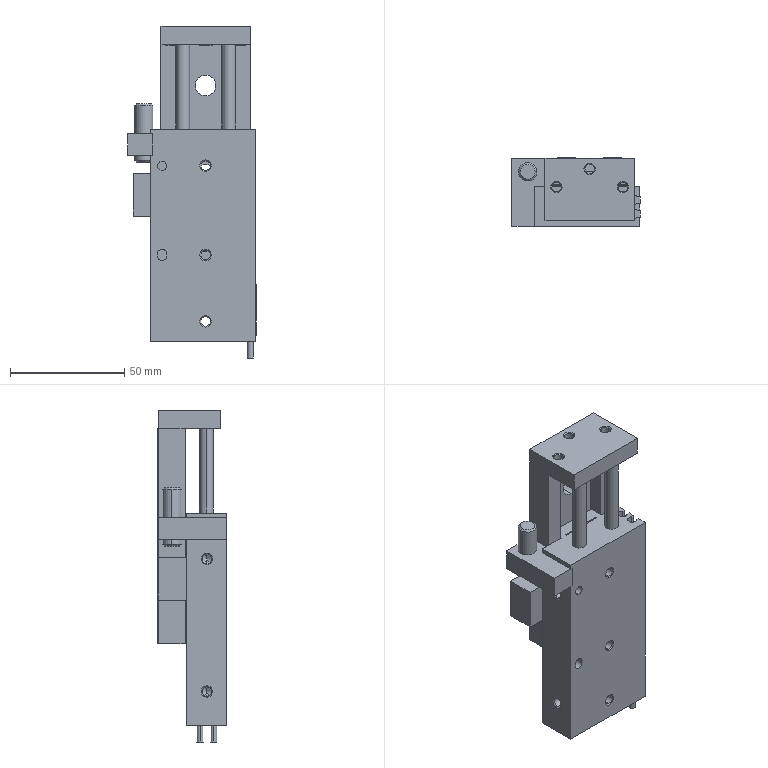Part | STEP file | 1105WWMXQ12-40CSP-M9NL(35)527 | 1 solid | 272 faces | box 56.1 x 30 x 145 mm | volume 123315 mm3 | plane 96 | cylinder 86 | cone 82 | spline 8 | commonest cylinder face diameters 3.24 x32 4 x14 4.13 x10 4.2 x6 9 x6 2.7 x4